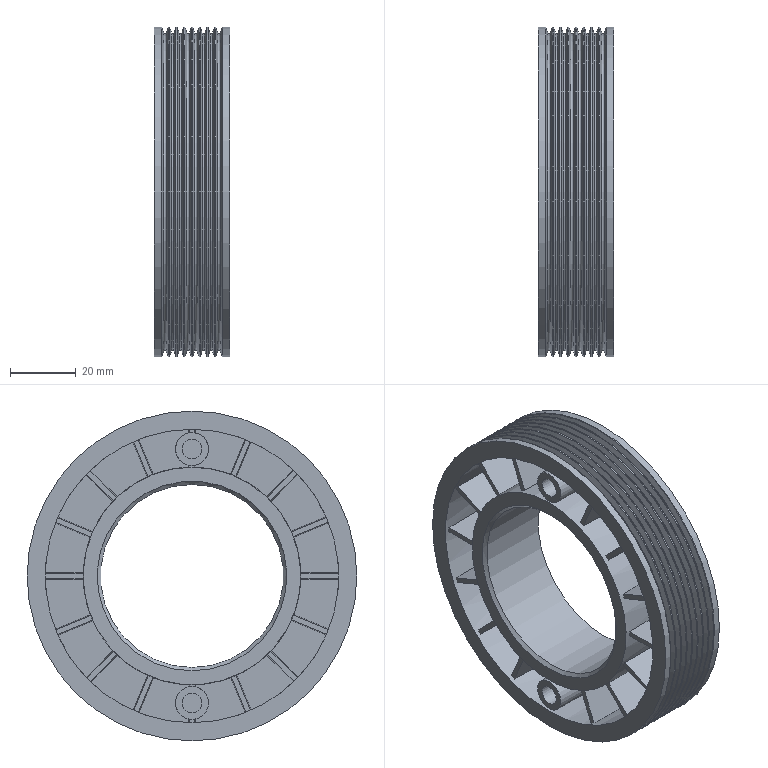Part | STEP file | PN_0017_default | 1 solid | 120 faces | box 23 x 100 x 100 mm | volume 79245 mm3 | plane 77 | torus 17 | cone 17 | cylinder 9 | commonest cylinder face diameters 6 x2 10 x2 100 x2 55.5 x1 66 x1 89 x1